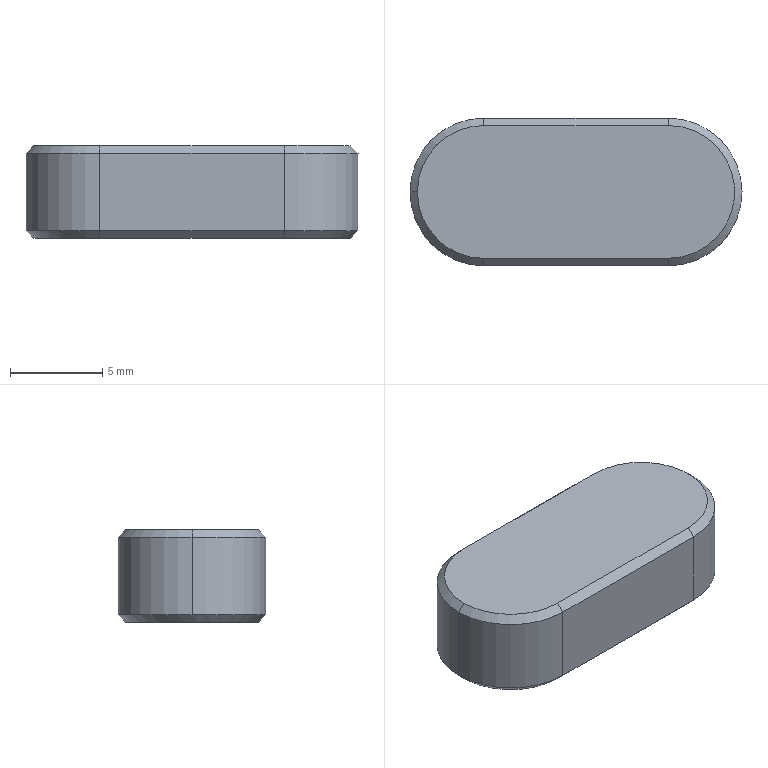Part | SolidWorks | features BaseBody 1 | 1 solid | 17 faces | box 18 x 8 x 5 mm | volume 644.24 mm3 | plane 8 | cone 6 | cylinder 3 | commonest cylinder face diameters 8 x3
STEP:
#1=CARTESIAN_POINT('',(14.,-3.6,-3.));
#2=VERTEX_POINT('',#1);
#3=CARTESIAN_POINT('',(17.6,0.,-3.));
#4=VERTEX_POINT('',#3);
#5=CARTESIAN_POINT('',(14.,0.,-3.));
#6=DIRECTION('',(0.,0.,1.));
#7=DIRECTION('',(1.,0.,0.));
#8=AXIS2_PLACEMENT_3D('',#5,#6,#7);
#9=CIRCLE('',#8,3.6);
#10=EDGE_CURVE('',#2,#4,#9,.T.);
#11=ORIENTED_EDGE('',*,*,#10,.T.);
#12=CARTESIAN_POINT('',(18.,0.,-2.6));
#13=VERTEX_POINT('',#12);
#14=CARTESIAN_POINT('',(18.,0.,-2.6));
#15=DIRECTION('',(0.7071,0.,0.7071));
#16=VECTOR('',#15,1000.);
#17=LINE('',#14,#16);
#18=EDGE_CURVE('',#4,#13,#17,.T.);
#19=ORIENTED_EDGE('',*,*,#18,.T.);
#20=CARTESIAN_POINT('',(14.,-4.,-2.6));
#21=VERTEX_POINT('',#20);
#22=CARTESIAN_POINT('',(14.,0.,-2.6));
#23=DIRECTION('',(0.,0.,-1.));
#24=DIRECTION('',(0.,1.,0.));
#25=AXIS2_PLACEMENT_3D('',#22,#23,#24);
#26=CIRCLE('',#25,4.);
#27=EDGE_CURVE('',#13,#21,#26,.T.);
#28=ORIENTED_EDGE('',*,*,#27,.T.);
#29=CARTESIAN_POINT('',(14.,-3.8,-2.8));
#30=DIRECTION('',(0.,-0.7071,0.7071));
#31=VECTOR('',#30,1000.);
#32=LINE('',#29,#31);
#33=EDGE_CURVE('',#2,#21,#32,.T.);
#34=ORIENTED_EDGE('',*,*,#33,.F.);
#35=EDGE_LOOP('',(#11,#19,#28,#34));
#36=FACE_OUTER_BOUND('',#35,.T.);
#37=CARTESIAN_POINT('',(14.,0.,-2.6));
#38=DIRECTION('',(0.,0.,1.));
#39=DIRECTION('',(1.,0.,0.));
#40=AXIS2_PLACEMENT_3D('',#37,#38,#39);
#41=CONICAL_SURFACE('',#40,4.,0.7854);
#42=ADVANCED_FACE('',(#36),#41,.T.);
#43=CARTESIAN_POINT('',(4.,-4.,1.6));
#44=VERTEX_POINT('',#43);
#45=CARTESIAN_POINT('',(0.,0.,1.6));
#46=VERTEX_POINT('',#45);
#47=CARTESIAN_POINT('',(4.,0.,1.6));
#48=DIRECTION('',(0.,0.,-1.));
#49=DIRECTION('',(-1.,0.,0.));
#50=AXIS2_PLACEMENT_3D('',#47,#48,#49);
#51=CIRCLE('',#50,4.);
#52=EDGE_CURVE('',#44,#46,#51,.T.);
#53=ORIENTED_EDGE('',*,*,#52,.T.);
#54=CARTESIAN_POINT('',(0.,0.,-2.6));
#55=VERTEX_POINT('',#54);
#56=CARTESIAN_POINT('',(0.,0.,0.));
#57=DIRECTION('',(0.,0.,-1.));
#58=VECTOR('',#57,1000.);
#59=LINE('',#56,#58);
#60=EDGE_CURVE('',#46,#55,#59,.T.);
#61=ORIENTED_EDGE('',*,*,#60,.T.);
#62=CARTESIAN_POINT('',(4.,-4.,-2.6));
#63=VERTEX_POINT('',#62);
#64=CARTESIAN_POINT('',(4.,0.,-2.6));
#65=DIRECTION('',(0.,0.,-1.));
#66=DIRECTION('',(0.,-1.,0.));
#67=AXIS2_PLACEMENT_3D('',#64,#65,#66);
#68=CIRCLE('',#67,4.);
#69=EDGE_CURVE('',#63,#55,#68,.T.);
#70=ORIENTED_EDGE('',*,*,#69,.F.);
#71=CARTESIAN_POINT('',(4.,-4.,0.));
#72=DIRECTION('',(0.,0.,-1.));
#73=VECTOR('',#72,1000.);
#74=LINE('',#71,#73);
#75=EDGE_CURVE('',#44,#63,#74,.T.);
#76=ORIENTED_EDGE('',*,*,#75,.F.);
#77=EDGE_LOOP('',(#53,#61,#70,#76));
#78=FACE_OUTER_BOUND('',#77,.T.);
#79=CARTESIAN_POINT('',(4.,0.,0.));
#80=DIRECTION('',(0.,0.,-1.));
#81=DIRECTION('',(-1.,0.,0.));
#82=AXIS2_PLACEMENT_3D('',#79,#80,#81);
#83=CYLINDRICAL_SURFACE('',#82,4.);
#84=ADVANCED_FACE('',(#78),#83,.T.);
#85=CARTESIAN_POINT('',(4.,-3.6,2.));
#86=VERTEX_POINT('',#85);
#87=CARTESIAN_POINT('',(0.4,0.,2.));
#88=VERTEX_POINT('',#87);
#89=CARTESIAN_POINT('',(4.,0.,2.));
#90=DIRECTION('',(0.,0.,-1.));
#91=DIRECTION('',(-1.,0.,0.));
#92=AXIS2_PLACEMENT_3D('',#89,#90,#91);
#93=CIRCLE('',#92,3.6);
#94=EDGE_CURVE('',#86,#88,#93,.T.);
#95=ORIENTED_EDGE('',*,*,#94,.T.);
#96=CARTESIAN_POINT('',(0.,0.,1.6));
#97=DIRECTION('',(-0.7071,0.,-0.7071));
#98=VECTOR('',#97,1000.);
#99=LINE('',#96,#98);
#100=EDGE_CURVE('',#88,#46,#99,.T.);
#101=ORIENTED_EDGE('',*,*,#100,.T.);
#102=ORIENTED_EDGE('',*,*,#52,.F.);
#103=CARTESIAN_POINT('',(4.,-3.8,1.8));
#104=DIRECTION('',(0.,-0.7071,-0.7071));
#105=VECTOR('',#104,1000.);
#106=LINE('',#103,#105);
#107=EDGE_CURVE('',#86,#44,#106,.T.);
#108=ORIENTED_EDGE('',*,*,#107,.F.);
#109=EDGE_LOOP('',(#95,#101,#102,#108));
#110=FACE_OUTER_BOUND('',#109,.T.);
#111=CARTESIAN_POINT('',(4.,0.,1.6));
#112=DIRECTION('',(0.,0.,-1.));
#113=DIRECTION('',(-1.,0.,0.));
#114=AXIS2_PLACEMENT_3D('',#111,#112,#113);
#115=CONICAL_SURFACE('',#114,4.,0.7854);
#116=ADVANCED_FACE('',(#110),#115,.T.);
#117=CARTESIAN_POINT('',(4.,3.6,-3.));
#118=VERTEX_POINT('',#117);
#119=CARTESIAN_POINT('',(4.,-3.6,-3.));
#120=VERTEX_POINT('',#119);
#121=CARTESIAN_POINT('',(4.,0.,-3.));
#122=DIRECTION('',(0.,0.,1.));
#123=DIRECTION('',(1.,0.,0.));
#124=AXIS2_PLACEMENT_3D('',#121,#122,#123);
#125=CIRCLE('',#124,3.6);
#126=EDGE_CURVE('',#118,#120,#125,.T.);
#127=ORIENTED_EDGE('',*,*,#126,.F.);
#128=CARTESIAN_POINT('',(14.,3.6,-3.));
#129=VERTEX_POINT('',#128);
#130=CARTESIAN_POINT('',(9.,3.6,-3.));
#131=DIRECTION('',(-1.,0.,0.));
#132=VECTOR('',#131,1000.);
#133=LINE('',#130,#132);
#134=EDGE_CURVE('',#129,#118,#133,.T.);
#135=ORIENTED_EDGE('',*,*,#134,.F.);
#136=CARTESIAN_POINT('',(14.,0.,-3.));
#137=DIRECTION('',(0.,0.,1.));
#138=DIRECTION('',(1.,0.,0.));
#139=AXIS2_PLACEMENT_3D('',#136,#137,#138);
#140=CIRCLE('',#139,3.6);
#141=EDGE_CURVE('',#4,#129,#140,.T.);
#142=ORIENTED_EDGE('',*,*,#141,.F.);
#143=ORIENTED_EDGE('',*,*,#10,.F.);
#144=CARTESIAN_POINT('',(9.,-3.6,-3.));
#145=DIRECTION('',(1.,0.,0.));
#146=VECTOR('',#145,1000.);
#147=LINE('',#144,#146);
#148=EDGE_CURVE('',#120,#2,#147,.T.);
#149=ORIENTED_EDGE('',*,*,#148,.F.);
#150=EDGE_LOOP('',(#127,#135,#142,#143,#149));
#151=FACE_OUTER_BOUND('',#150,.T.);
#152=CARTESIAN_POINT('',(9.,0.,-3.));
#153=DIRECTION('',(0.,0.,1.));
#154=DIRECTION('',(1.,0.,0.));
#155=AXIS2_PLACEMENT_3D('',#152,#153,#154);
#156=PLANE('',#155);
#157=ADVANCED_FACE('',(#151),#156,.F.);
#158=CARTESIAN_POINT('',(4.,-3.8,-2.8));
#159=DIRECTION('',(0.,0.7071,-0.7071));
#160=VECTOR('',#159,1000.);
#161=LINE('',#158,#160);
#162=EDGE_CURVE('',#63,#120,#161,.T.);
#163=ORIENTED_EDGE('',*,*,#162,.T.);
#164=ORIENTED_EDGE('',*,*,#148,.T.);
#165=ORIENTED_EDGE('',*,*,#33,.T.);
#166=CARTESIAN_POINT('',(6.5,-4.,-2.6));
#167=DIRECTION('',(-1.,0.,0.));
#168=VECTOR('',#167,1000.);
#169=LINE('',#166,#168);
#170=EDGE_CURVE('',#21,#63,#169,.T.);
#171=ORIENTED_EDGE('',*,*,#170,.T.);
#172=EDGE_LOOP('',(#163,#164,#165,#171));
#173=FACE_OUTER_BOUND('',#172,.T.);
#174=CARTESIAN_POINT('',(6.5,-3.8,-2.8));
#175=DIRECTION('',(0.,-0.7071,-0.7071));
#176=DIRECTION('',(0.,0.7071,-0.7071));
#177=AXIS2_PLACEMENT_3D('',#174,#175,#176);
#178=PLANE('',#177);
#179=ADVANCED_FACE('',(#173),#178,.T.);
#180=ORIENTED_EDGE('',*,*,#162,.F.);
#181=ORIENTED_EDGE('',*,*,#69,.T.);
#182=CARTESIAN_POINT('',(4.,4.,-2.6));
#183=VERTEX_POINT('',#182);
#184=CARTESIAN_POINT('',(4.,0.,-2.6));
#185=DIRECTION('',(0.,0.,-1.));
#186=DIRECTION('',(0.,-1.,0.));
#187=AXIS2_PLACEMENT_3D('',#184,#185,#186);
#188=CIRCLE('',#187,4.);
#189=EDGE_CURVE('',#55,#183,#188,.T.);
#190=ORIENTED_EDGE('',*,*,#189,.T.);
#191=CARTESIAN_POINT('',(4.,499000.,498993.4));
#192=DIRECTION('',(0.,-0.7071,-0.7071));
#193=VECTOR('',#192,1000.);
#194=LINE('',#191,#193);
#195=EDGE_CURVE('',#183,#118,#194,.T.);
#196=ORIENTED_EDGE('',*,*,#195,.T.);
#197=ORIENTED_EDGE('',*,*,#126,.T.);
#198=EDGE_LOOP('',(#180,#181,#190,#196,#197));
#199=FACE_OUTER_BOUND('',#198,.T.);
#200=CARTESIAN_POINT('',(4.,0.,-2.6));
#201=DIRECTION('',(0.,0.,1.));
#202=DIRECTION('',(1.,0.,0.));
#203=AXIS2_PLACEMENT_3D('',#200,#201,#202);
#204=CONICAL_SURFACE('',#203,4.,0.7854);
#205=ADVANCED_FACE('',(#199),#204,.T.);
#206=ORIENTED_EDGE('',*,*,#195,.F.);
#207=CARTESIAN_POINT('',(14.,4.,-2.6));
#208=VERTEX_POINT('',#207);
#209=CARTESIAN_POINT('',(11.5,4.,-2.6));
#210=DIRECTION('',(1.,0.,0.));
#211=VECTOR('',#210,1000.);
#212=LINE('',#209,#211);
#213=EDGE_CURVE('',#183,#208,#212,.T.);
#214=ORIENTED_EDGE('',*,*,#213,.T.);
#215=CARTESIAN_POINT('',(14.,3.8,-2.8));
#216=DIRECTION('',(0.,-0.7071,-0.7071));
#217=VECTOR('',#216,1000.);
#218=LINE('',#215,#217);
#219=EDGE_CURVE('',#208,#129,#218,.T.);
#220=ORIENTED_EDGE('',*,*,#219,.T.);
#221=ORIENTED_EDGE('',*,*,#134,.T.);
#222=EDGE_LOOP('',(#206,#214,#220,#221));
#223=FACE_OUTER_BOUND('',#222,.T.);
#224=CARTESIAN_POINT('',(11.5,3.8,-2.8));
#225=DIRECTION('',(0.,0.7071,-0.7071));
#226=DIRECTION('',(0.,0.7071,0.7071));
#227=AXIS2_PLACEMENT_3D('',#224,#225,#226);
#228=PLANE('',#227);
#229=ADVANCED_FACE('',(#223),#228,.T.);
#230=ORIENTED_EDGE('',*,*,#18,.F.);
#231=ORIENTED_EDGE('',*,*,#141,.T.);
#232=ORIENTED_EDGE('',*,*,#219,.F.);
#233=CARTESIAN_POINT('',(14.,0.,-2.6));
#234=DIRECTION('',(0.,0.,-1.));
#235=DIRECTION('',(0.,1.,0.));
#236=AXIS2_PLACEMENT_3D('',#233,#234,#235);
#237=CIRCLE('',#236,4.);
#238=EDGE_CURVE('',#208,#13,#237,.T.);
#239=ORIENTED_EDGE('',*,*,#238,.T.);
#240=EDGE_LOOP('',(#230,#231,#232,#239));
#241=FACE_OUTER_BOUND('',#240,.T.);
#242=CARTESIAN_POINT('',(14.,0.,-2.6));
#243=DIRECTION('',(0.,0.,1.));
#244=DIRECTION('',(1.,0.,0.));
#245=AXIS2_PLACEMENT_3D('',#242,#243,#244);
#246=CONICAL_SURFACE('',#245,4.,0.7854);
#247=ADVANCED_FACE('',(#241),#246,.T.);
#248=CARTESIAN_POINT('',(14.,-4.,1.6));
#249=VERTEX_POINT('',#248);
#250=CARTESIAN_POINT('',(4.,-4.,1.6));
#251=DIRECTION('',(-1.,0.,0.));
#252=VECTOR('',#251,1000.);
#253=LINE('',#250,#252);
#254=EDGE_CURVE('',#249,#44,#253,.T.);
#255=ORIENTED_EDGE('',*,*,#254,.T.);
#256=ORIENTED_EDGE('',*,*,#75,.T.);
#257=ORIENTED_EDGE('',*,*,#170,.F.);
#258=CARTESIAN_POINT('',(14.,-4.,0.));
#259=DIRECTION('',(0.,0.,1.));
#260=VECTOR('',#259,1000.);
#261=LINE('',#258,#260);
#262=EDGE_CURVE('',#21,#249,#261,.T.);
#263=ORIENTED_EDGE('',*,*,#262,.T.);
#264=EDGE_LOOP('',(#255,#256,#257,#263));
#265=FACE_OUTER_BOUND('',#264,.T.);
#266=CARTESIAN_POINT('',(4.,-4.,0.));
#267=DIRECTION('',(0.,-1.,0.));
#268=DIRECTION('',(1.,0.,0.));
#269=AXIS2_PLACEMENT_3D('',#266,#267,#268);
#270=PLANE('',#269);
#271=ADVANCED_FACE('',(#265),#270,.T.);
#272=ORIENTED_EDGE('',*,*,#60,.F.);
#273=CARTESIAN_POINT('',(4.,4.,1.6));
#274=VERTEX_POINT('',#273);
#275=CARTESIAN_POINT('',(4.,0.,1.6));
#276=DIRECTION('',(0.,0.,-1.));
#277=DIRECTION('',(-1.,0.,0.));
#278=AXIS2_PLACEMENT_3D('',#275,#276,#277);
#279=CIRCLE('',#278,4.);
#280=EDGE_CURVE('',#46,#274,#279,.T.);
#281=ORIENTED_EDGE('',*,*,#280,.T.);
#282=CARTESIAN_POINT('',(4.,4.,0.));
#283=DIRECTION('',(0.,0.,-1.));
#284=VECTOR('',#283,1000.);
#285=LINE('',#282,#284);
#286=EDGE_CURVE('',#274,#183,#285,.T.);
#287=ORIENTED_EDGE('',*,*,#286,.T.);
#288=ORIENTED_EDGE('',*,*,#189,.F.);
#289=EDGE_LOOP('',(#272,#281,#287,#288));
#290=FACE_OUTER_BOUND('',#289,.T.);
#291=CARTESIAN_POINT('',(4.,0.,0.));
#292=DIRECTION('',(0.,0.,-1.));
#293=DIRECTION('',(-1.,0.,0.));
#294=AXIS2_PLACEMENT_3D('',#291,#292,#293);
#295=CYLINDRICAL_SURFACE('',#294,4.);
#296=ADVANCED_FACE('',(#290),#295,.T.);
#297=CARTESIAN_POINT('',(14.,4.,1.6));
#298=VERTEX_POINT('',#297);
#299=CARTESIAN_POINT('',(14.,4.,1.6));
#300=DIRECTION('',(1.,0.,0.));
#301=VECTOR('',#300,1000.);
#302=LINE('',#299,#301);
#303=EDGE_CURVE('',#274,#298,#302,.T.);
#304=ORIENTED_EDGE('',*,*,#303,.T.);
#305=CARTESIAN_POINT('',(14.,4.,0.));
#306=DIRECTION('',(0.,0.,-1.));
#307=VECTOR('',#306,1000.);
#308=LINE('',#305,#307);
#309=EDGE_CURVE('',#298,#208,#308,.T.);
#310=ORIENTED_EDGE('',*,*,#309,.T.);
#311=ORIENTED_EDGE('',*,*,#213,.F.);
#312=ORIENTED_EDGE('',*,*,#286,.F.);
#313=EDGE_LOOP('',(#304,#310,#311,#312));
#314=FACE_OUTER_BOUND('',#313,.T.);
#315=CARTESIAN_POINT('',(14.,4.,0.));
#316=DIRECTION('',(0.,1.,0.));
#317=DIRECTION('',(0.,0.,1.));
#318=AXIS2_PLACEMENT_3D('',#315,#316,#317);
#319=PLANE('',#318);
#320=ADVANCED_FACE('',(#314),#319,.T.);
#321=CARTESIAN_POINT('',(14.,0.,1.6));
#322=DIRECTION('',(0.,0.,-1.));
#323=DIRECTION('',(-1.,0.,0.));
#324=AXIS2_PLACEMENT_3D('',#321,#322,#323);
#325=CIRCLE('',#324,4.);
#326=EDGE_CURVE('',#298,#249,#325,.T.);
#327=ORIENTED_EDGE('',*,*,#326,.T.);
#328=ORIENTED_EDGE('',*,*,#262,.F.);
#329=ORIENTED_EDGE('',*,*,#27,.F.);
#330=ORIENTED_EDGE('',*,*,#238,.F.);
#331=ORIENTED_EDGE('',*,*,#309,.F.);
#332=EDGE_LOOP('',(#327,#328,#329,#330,#331));
#333=FACE_OUTER_BOUND('',#332,.T.);
#334=CARTESIAN_POINT('',(14.,0.,0.));
#335=DIRECTION('',(0.,0.,-1.));
#336=DIRECTION('',(-1.,0.,0.));
#337=AXIS2_PLACEMENT_3D('',#334,#335,#336);
#338=CYLINDRICAL_SURFACE('',#337,4.);
#339=ADVANCED_FACE('',(#333),#338,.T.);
#340=ORIENTED_EDGE('',*,*,#107,.T.);
#341=ORIENTED_EDGE('',*,*,#254,.F.);
#342=CARTESIAN_POINT('',(14.,-3.6,2.));
#343=VERTEX_POINT('',#342);
#344=CARTESIAN_POINT('',(14.,-3.8,1.8));
#345=DIRECTION('',(0.,0.7071,0.7071));
#346=VECTOR('',#345,1000.);
#347=LINE('',#344,#346);
#348=EDGE_CURVE('',#249,#343,#347,.T.);
#349=ORIENTED_EDGE('',*,*,#348,.T.);
#350=CARTESIAN_POINT('',(6.5,-3.6,2.));
#351=DIRECTION('',(-1.,0.,0.));
#352=VECTOR('',#351,1000.);
#353=LINE('',#350,#352);
#354=EDGE_CURVE('',#343,#86,#353,.T.);
#355=ORIENTED_EDGE('',*,*,#354,.T.);
#356=EDGE_LOOP('',(#340,#341,#349,#355));
#357=FACE_OUTER_BOUND('',#356,.T.);
#358=CARTESIAN_POINT('',(6.5,-3.8,1.8));
#359=DIRECTION('',(0.,-0.7071,0.7071));
#360=DIRECTION('',(0.,-0.7071,-0.7071));
#361=AXIS2_PLACEMENT_3D('',#358,#359,#360);
#362=PLANE('',#361);
#363=ADVANCED_FACE('',(#357),#362,.T.);
#364=ORIENTED_EDGE('',*,*,#100,.F.);
#365=CARTESIAN_POINT('',(4.,3.6,2.));
#366=VERTEX_POINT('',#365);
#367=CARTESIAN_POINT('',(4.,0.,2.));
#368=DIRECTION('',(0.,0.,-1.));
#369=DIRECTION('',(-1.,0.,0.));
#370=AXIS2_PLACEMENT_3D('',#367,#368,#369);
#371=CIRCLE('',#370,3.6);
#372=EDGE_CURVE('',#88,#366,#371,.T.);
#373=ORIENTED_EDGE('',*,*,#372,.T.);
#374=CARTESIAN_POINT('',(4.,499000.,-498994.4));
#375=DIRECTION('',(0.,0.7071,-0.7071));
#376=VECTOR('',#375,1000.);
#377=LINE('',#374,#376);
#378=EDGE_CURVE('',#366,#274,#377,.T.);
#379=ORIENTED_EDGE('',*,*,#378,.T.);
#380=ORIENTED_EDGE('',*,*,#280,.F.);
#381=EDGE_LOOP('',(#364,#373,#379,#380));
#382=FACE_OUTER_BOUND('',#381,.T.);
#383=CARTESIAN_POINT('',(4.,0.,1.6));
#384=DIRECTION('',(0.,0.,-1.));
#385=DIRECTION('',(-1.,0.,0.));
#386=AXIS2_PLACEMENT_3D('',#383,#384,#385);
#387=CONICAL_SURFACE('',#386,4.,0.7854);
#388=ADVANCED_FACE('',(#382),#387,.T.);
#389=ORIENTED_EDGE('',*,*,#378,.F.);
#390=CARTESIAN_POINT('',(14.,3.6,2.));
#391=VERTEX_POINT('',#390);
#392=CARTESIAN_POINT('',(11.5,3.6,2.));
#393=DIRECTION('',(1.,0.,0.));
#394=VECTOR('',#393,1000.);
#395=LINE('',#392,#394);
#396=EDGE_CURVE('',#366,#391,#395,.T.);
#397=ORIENTED_EDGE('',*,*,#396,.T.);
#398=CARTESIAN_POINT('',(14.,3.8,1.8));
#399=DIRECTION('',(0.,0.7071,-0.7071));
#400=VECTOR('',#399,1000.);
#401=LINE('',#398,#400);
#402=EDGE_CURVE('',#391,#298,#401,.T.);
#403=ORIENTED_EDGE('',*,*,#402,.T.);
#404=ORIENTED_EDGE('',*,*,#303,.F.);
#405=EDGE_LOOP('',(#389,#397,#403,#404));
#406=FACE_OUTER_BOUND('',#405,.T.);
#407=CARTESIAN_POINT('',(11.5,3.8,1.8));
#408=DIRECTION('',(0.,0.7071,0.7071));
#409=DIRECTION('',(0.,-0.7071,0.7071));
#410=AXIS2_PLACEMENT_3D('',#407,#408,#409);
#411=PLANE('',#410);
#412=ADVANCED_FACE('',(#406),#411,.T.);
#413=ORIENTED_EDGE('',*,*,#402,.F.);
#414=CARTESIAN_POINT('',(14.,0.,2.));
#415=DIRECTION('',(0.,0.,-1.));
#416=DIRECTION('',(-1.,0.,0.));
#417=AXIS2_PLACEMENT_3D('',#414,#415,#416);
#418=CIRCLE('',#417,3.6);
#419=EDGE_CURVE('',#391,#343,#418,.T.);
#420=ORIENTED_EDGE('',*,*,#419,.T.);
#421=ORIENTED_EDGE('',*,*,#348,.F.);
#422=ORIENTED_EDGE('',*,*,#326,.F.);
#423=EDGE_LOOP('',(#413,#420,#421,#422));
#424=FACE_OUTER_BOUND('',#423,.T.);
#425=CARTESIAN_POINT('',(14.,0.,1.6));
#426=DIRECTION('',(0.,0.,-1.));
#427=DIRECTION('',(-1.,0.,0.));
#428=AXIS2_PLACEMENT_3D('',#425,#426,#427);
#429=CONICAL_SURFACE('',#428,4.,0.7854);
#430=ADVANCED_FACE('',(#424),#429,.T.);
#431=ORIENTED_EDGE('',*,*,#419,.F.);
#432=ORIENTED_EDGE('',*,*,#396,.F.);
#433=ORIENTED_EDGE('',*,*,#372,.F.);
#434=ORIENTED_EDGE('',*,*,#94,.F.);
#435=ORIENTED_EDGE('',*,*,#354,.F.);
#436=EDGE_LOOP('',(#431,#432,#433,#434,#435));
#437=FACE_OUTER_BOUND('',#436,.T.);
#438=CARTESIAN_POINT('',(9.,0.,2.));
#439=DIRECTION('',(0.,0.,1.));
#440=DIRECTION('',(1.,0.,0.));
#441=AXIS2_PLACEMENT_3D('',#438,#439,#440);
#442=PLANE('',#441);
#443=ADVANCED_FACE('',(#437),#442,.T.);
#444=CLOSED_SHELL('',(#42,#84,#116,#157,#179,#205,#229,#247,#271,#296,#320,#339,#363,#388,#412,#430,#443));
#445=MANIFOLD_SOLID_BREP('',#444);
#446=CARTESIAN_POINT('',(0.,0.,0.));
#447=DIRECTION('',(0.,0.,1.));
#448=DIRECTION('',(1.,0.,0.));
#449=AXIS2_PLACEMENT_3D('',#446,#447,#448);
#450=(LENGTH_UNIT()NAMED_UNIT(*)SI_UNIT(.MILLI.,.METRE.));
#451=UNCERTAINTY_MEASURE_WITH_UNIT(LENGTH_MEASURE(0.00001),#450,'','');
#452=(NAMED_UNIT(*)PLANE_ANGLE_UNIT()SI_UNIT($,.RADIAN.));
#453=(NAMED_UNIT(*)SI_UNIT($,.STERADIAN.)SOLID_ANGLE_UNIT());
#454=(GEOMETRIC_REPRESENTATION_CONTEXT(3)GLOBAL_UNCERTAINTY_ASSIGNED_CONTEXT((#451))GLOBAL_UNIT_ASSIGNED_CONTEXT((#450,#452,#453))REPRESENTATION_CONTEXT('',''));
#455=ADVANCED_BREP_SHAPE_REPRESENTATION('',(#445,#449),#454);